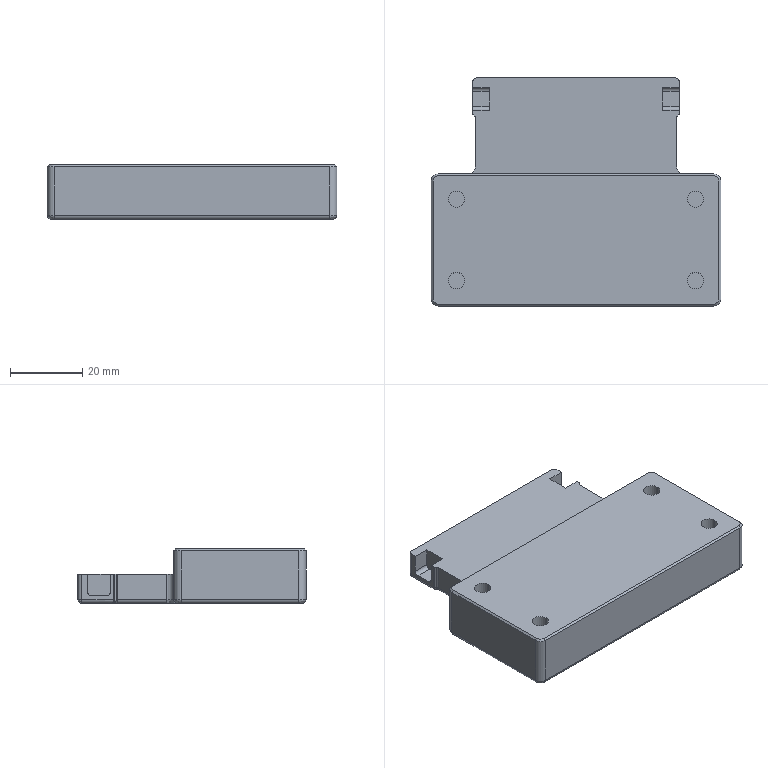Part | SolidWorks | features BaseBody 1 | 1 solid | 226 faces | box 80 x 63 x 15 mm | volume 53710 mm3 | plane 113 | cylinder 76 | spline 33 | cone 4 | commonest cylinder face diameters 2 x18 4.5 x10 7 x8 8 x8 4 x6 1 x4